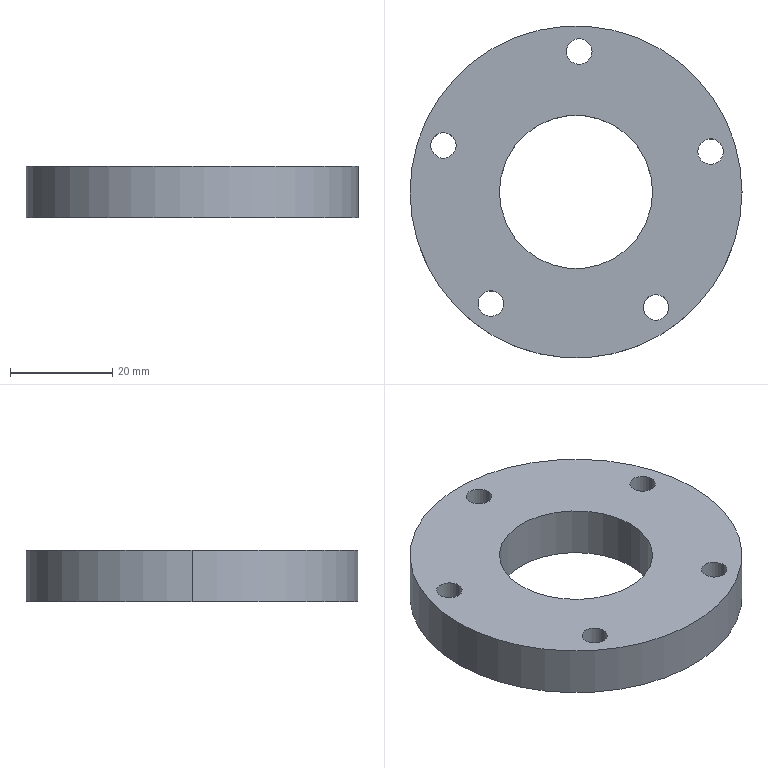Part | SolidWorks | features BaseBody 1 | 1 solid | 16 faces | box 65 x 65 x 10 mm | volume 25133 mm3 | cylinder 14 | plane 2 | commonest cylinder face diameters 5 x10 30 x2 65 x2
STEP:
#1=CARTESIAN_POINT('',(-23.45,9.102,10.));
#2=VERTEX_POINT('',#1);
#3=CARTESIAN_POINT('',(-28.45,9.102,10.));
#4=VERTEX_POINT('',#3);
#5=CARTESIAN_POINT('',(-25.95,9.102,10.));
#6=DIRECTION('',(0.,0.,-1.));
#7=DIRECTION('',(-1.,0.,0.));
#8=AXIS2_PLACEMENT_3D('',#5,#6,#7);
#9=CIRCLE('',#8,2.5);
#10=EDGE_CURVE('',#2,#4,#9,.T.);
#11=ORIENTED_EDGE('',*,*,#10,.F.);
#12=CARTESIAN_POINT('',(-23.45,9.102,0.));
#13=VERTEX_POINT('',#12);
#14=CARTESIAN_POINT('',(-23.45,9.102,10.));
#15=DIRECTION('',(0.,0.,-1.));
#16=VECTOR('',#15,1000.);
#17=LINE('',#14,#16);
#18=EDGE_CURVE('',#2,#13,#17,.T.);
#19=ORIENTED_EDGE('',*,*,#18,.T.);
#20=CARTESIAN_POINT('',(-28.45,9.102,0.));
#21=VERTEX_POINT('',#20);
#22=CARTESIAN_POINT('',(-25.95,9.102,0.));
#23=DIRECTION('',(0.,0.,1.));
#24=DIRECTION('',(-1.,0.,0.));
#25=AXIS2_PLACEMENT_3D('',#22,#23,#24);
#26=CIRCLE('',#25,2.5);
#27=EDGE_CURVE('',#21,#13,#26,.T.);
#28=ORIENTED_EDGE('',*,*,#27,.F.);
#29=CARTESIAN_POINT('',(-28.45,9.102,10.));
#30=DIRECTION('',(0.,0.,-1.));
#31=VECTOR('',#30,1000.);
#32=LINE('',#29,#31);
#33=EDGE_CURVE('',#4,#21,#32,.T.);
#34=ORIENTED_EDGE('',*,*,#33,.F.);
#35=EDGE_LOOP('',(#11,#19,#28,#34));
#36=FACE_OUTER_BOUND('',#35,.T.);
#37=CARTESIAN_POINT('',(-25.95,9.102,10.));
#38=DIRECTION('',(0.,0.,-1.));
#39=DIRECTION('',(-1.,0.,0.));
#40=AXIS2_PLACEMENT_3D('',#37,#38,#39);
#41=CYLINDRICAL_SURFACE('',#40,2.5);
#42=ADVANCED_FACE('',(#36),#41,.F.);
#43=CARTESIAN_POINT('',(18.144,-22.616,10.));
#44=VERTEX_POINT('',#43);
#45=CARTESIAN_POINT('',(13.144,-22.616,10.));
#46=VERTEX_POINT('',#45);
#47=CARTESIAN_POINT('',(15.644,-22.616,10.));
#48=DIRECTION('',(0.,0.,-1.));
#49=DIRECTION('',(-1.,0.,0.));
#50=AXIS2_PLACEMENT_3D('',#47,#48,#49);
#51=CIRCLE('',#50,2.5);
#52=EDGE_CURVE('',#44,#46,#51,.T.);
#53=ORIENTED_EDGE('',*,*,#52,.F.);
#54=CARTESIAN_POINT('',(18.144,-22.616,0.));
#55=VERTEX_POINT('',#54);
#56=CARTESIAN_POINT('',(18.144,-22.616,10.));
#57=DIRECTION('',(0.,0.,-1.));
#58=VECTOR('',#57,1000.);
#59=LINE('',#56,#58);
#60=EDGE_CURVE('',#44,#55,#59,.T.);
#61=ORIENTED_EDGE('',*,*,#60,.T.);
#62=CARTESIAN_POINT('',(13.144,-22.616,0.));
#63=VERTEX_POINT('',#62);
#64=CARTESIAN_POINT('',(15.644,-22.616,0.));
#65=DIRECTION('',(0.,0.,1.));
#66=DIRECTION('',(-1.,0.,0.));
#67=AXIS2_PLACEMENT_3D('',#64,#65,#66);
#68=CIRCLE('',#67,2.5);
#69=EDGE_CURVE('',#63,#55,#68,.T.);
#70=ORIENTED_EDGE('',*,*,#69,.F.);
#71=CARTESIAN_POINT('',(13.144,-22.616,10.));
#72=DIRECTION('',(0.,0.,-1.));
#73=VECTOR('',#72,1000.);
#74=LINE('',#71,#73);
#75=EDGE_CURVE('',#46,#63,#74,.T.);
#76=ORIENTED_EDGE('',*,*,#75,.F.);
#77=EDGE_LOOP('',(#53,#61,#70,#76));
#78=FACE_OUTER_BOUND('',#77,.T.);
#79=CARTESIAN_POINT('',(15.644,-22.616,10.));
#80=DIRECTION('',(0.,0.,-1.));
#81=DIRECTION('',(-1.,0.,0.));
#82=AXIS2_PLACEMENT_3D('',#79,#80,#81);
#83=CYLINDRICAL_SURFACE('',#82,2.5);
#84=ADVANCED_FACE('',(#78),#83,.F.);
#85=CARTESIAN_POINT('',(3.137,27.493,10.));
#86=VERTEX_POINT('',#85);
#87=CARTESIAN_POINT('',(-1.863,27.493,10.));
#88=VERTEX_POINT('',#87);
#89=CARTESIAN_POINT('',(0.637,27.493,10.));
#90=DIRECTION('',(0.,0.,-1.));
#91=DIRECTION('',(-1.,0.,0.));
#92=AXIS2_PLACEMENT_3D('',#89,#90,#91);
#93=CIRCLE('',#92,2.5);
#94=EDGE_CURVE('',#86,#88,#93,.T.);
#95=ORIENTED_EDGE('',*,*,#94,.F.);
#96=CARTESIAN_POINT('',(3.137,27.493,0.));
#97=VERTEX_POINT('',#96);
#98=CARTESIAN_POINT('',(3.137,27.493,10.));
#99=DIRECTION('',(0.,0.,-1.));
#100=VECTOR('',#99,1000.);
#101=LINE('',#98,#100);
#102=EDGE_CURVE('',#86,#97,#101,.T.);
#103=ORIENTED_EDGE('',*,*,#102,.T.);
#104=CARTESIAN_POINT('',(-1.863,27.493,0.));
#105=VERTEX_POINT('',#104);
#106=CARTESIAN_POINT('',(0.637,27.493,0.));
#107=DIRECTION('',(0.,0.,1.));
#108=DIRECTION('',(-1.,0.,0.));
#109=AXIS2_PLACEMENT_3D('',#106,#107,#108);
#110=CIRCLE('',#109,2.5);
#111=EDGE_CURVE('',#105,#97,#110,.T.);
#112=ORIENTED_EDGE('',*,*,#111,.F.);
#113=CARTESIAN_POINT('',(-1.863,27.493,10.));
#114=DIRECTION('',(0.,0.,-1.));
#115=VECTOR('',#114,1000.);
#116=LINE('',#113,#115);
#117=EDGE_CURVE('',#88,#105,#116,.T.);
#118=ORIENTED_EDGE('',*,*,#117,.F.);
#119=EDGE_LOOP('',(#95,#103,#112,#118));
#120=FACE_OUTER_BOUND('',#119,.T.);
#121=CARTESIAN_POINT('',(0.637,27.493,10.));
#122=DIRECTION('',(0.,0.,-1.));
#123=DIRECTION('',(-1.,0.,0.));
#124=AXIS2_PLACEMENT_3D('',#121,#122,#123);
#125=CYLINDRICAL_SURFACE('',#124,2.5);
#126=ADVANCED_FACE('',(#120),#125,.F.);
#127=CARTESIAN_POINT('',(32.5,0.,10.));
#128=VERTEX_POINT('',#127);
#129=CARTESIAN_POINT('',(-32.5,0.,10.));
#130=VERTEX_POINT('',#129);
#131=CARTESIAN_POINT('',(0.,0.,10.));
#132=DIRECTION('',(0.,0.,1.));
#133=DIRECTION('',(-1.,0.,0.));
#134=AXIS2_PLACEMENT_3D('',#131,#132,#133);
#135=CIRCLE('',#134,32.5);
#136=EDGE_CURVE('',#128,#130,#135,.T.);
#137=ORIENTED_EDGE('',*,*,#136,.F.);
#138=CARTESIAN_POINT('',(32.5,0.,0.));
#139=VERTEX_POINT('',#138);
#140=CARTESIAN_POINT('',(32.5,0.,10.));
#141=DIRECTION('',(0.,0.,-1.));
#142=VECTOR('',#141,1000.);
#143=LINE('',#140,#142);
#144=EDGE_CURVE('',#128,#139,#143,.T.);
#145=ORIENTED_EDGE('',*,*,#144,.T.);
#146=CARTESIAN_POINT('',(-32.5,0.,0.));
#147=VERTEX_POINT('',#146);
#148=CARTESIAN_POINT('',(0.,0.,0.));
#149=DIRECTION('',(0.,0.,1.));
#150=DIRECTION('',(-1.,0.,0.));
#151=AXIS2_PLACEMENT_3D('',#148,#149,#150);
#152=CIRCLE('',#151,32.5);
#153=EDGE_CURVE('',#139,#147,#152,.T.);
#154=ORIENTED_EDGE('',*,*,#153,.T.);
#155=CARTESIAN_POINT('',(-32.5,0.,10.));
#156=DIRECTION('',(0.,0.,-1.));
#157=VECTOR('',#156,1000.);
#158=LINE('',#155,#157);
#159=EDGE_CURVE('',#130,#147,#158,.T.);
#160=ORIENTED_EDGE('',*,*,#159,.F.);
#161=EDGE_LOOP('',(#137,#145,#154,#160));
#162=FACE_OUTER_BOUND('',#161,.T.);
#163=CARTESIAN_POINT('',(0.,0.,10.));
#164=DIRECTION('',(0.,0.,-1.));
#165=DIRECTION('',(-1.,0.,0.));
#166=AXIS2_PLACEMENT_3D('',#163,#164,#165);
#167=CYLINDRICAL_SURFACE('',#166,32.5);
#168=ADVANCED_FACE('',(#162),#167,.T.);
#169=CARTESIAN_POINT('',(15.,0.,10.));
#170=VERTEX_POINT('',#169);
#171=CARTESIAN_POINT('',(-15.,0.,10.));
#172=VERTEX_POINT('',#171);
#173=CARTESIAN_POINT('',(0.,0.,10.));
#174=DIRECTION('',(0.,0.,-1.));
#175=DIRECTION('',(-1.,0.,0.));
#176=AXIS2_PLACEMENT_3D('',#173,#174,#175);
#177=CIRCLE('',#176,15.);
#178=EDGE_CURVE('',#170,#172,#177,.T.);
#179=ORIENTED_EDGE('',*,*,#178,.F.);
#180=CARTESIAN_POINT('',(15.,0.,0.));
#181=VERTEX_POINT('',#180);
#182=CARTESIAN_POINT('',(15.,0.,10.));
#183=DIRECTION('',(0.,0.,-1.));
#184=VECTOR('',#183,1000.);
#185=LINE('',#182,#184);
#186=EDGE_CURVE('',#170,#181,#185,.T.);
#187=ORIENTED_EDGE('',*,*,#186,.T.);
#188=CARTESIAN_POINT('',(-15.,0.,0.));
#189=VERTEX_POINT('',#188);
#190=CARTESIAN_POINT('',(0.,0.,0.));
#191=DIRECTION('',(0.,0.,1.));
#192=DIRECTION('',(-1.,0.,0.));
#193=AXIS2_PLACEMENT_3D('',#190,#191,#192);
#194=CIRCLE('',#193,15.);
#195=EDGE_CURVE('',#189,#181,#194,.T.);
#196=ORIENTED_EDGE('',*,*,#195,.F.);
#197=CARTESIAN_POINT('',(-15.,0.,10.));
#198=DIRECTION('',(0.,0.,-1.));
#199=VECTOR('',#198,1000.);
#200=LINE('',#197,#199);
#201=EDGE_CURVE('',#172,#189,#200,.T.);
#202=ORIENTED_EDGE('',*,*,#201,.F.);
#203=EDGE_LOOP('',(#179,#187,#196,#202));
#204=FACE_OUTER_BOUND('',#203,.T.);
#205=CARTESIAN_POINT('',(0.,0.,10.));
#206=DIRECTION('',(0.,0.,-1.));
#207=DIRECTION('',(-1.,0.,0.));
#208=AXIS2_PLACEMENT_3D('',#205,#206,#207);
#209=CYLINDRICAL_SURFACE('',#208,15.);
#210=ADVANCED_FACE('',(#204),#209,.F.);
#211=CARTESIAN_POINT('',(28.844,7.89,10.));
#212=VERTEX_POINT('',#211);
#213=CARTESIAN_POINT('',(23.844,7.89,10.));
#214=VERTEX_POINT('',#213);
#215=CARTESIAN_POINT('',(26.344,7.89,10.));
#216=DIRECTION('',(0.,0.,-1.));
#217=DIRECTION('',(-1.,0.,0.));
#218=AXIS2_PLACEMENT_3D('',#215,#216,#217);
#219=CIRCLE('',#218,2.5);
#220=EDGE_CURVE('',#212,#214,#219,.T.);
#221=ORIENTED_EDGE('',*,*,#220,.F.);
#222=CARTESIAN_POINT('',(28.844,7.89,0.));
#223=VERTEX_POINT('',#222);
#224=CARTESIAN_POINT('',(28.844,7.89,10.));
#225=DIRECTION('',(0.,0.,-1.));
#226=VECTOR('',#225,1000.);
#227=LINE('',#224,#226);
#228=EDGE_CURVE('',#212,#223,#227,.T.);
#229=ORIENTED_EDGE('',*,*,#228,.T.);
#230=CARTESIAN_POINT('',(23.844,7.89,0.));
#231=VERTEX_POINT('',#230);
#232=CARTESIAN_POINT('',(26.344,7.89,0.));
#233=DIRECTION('',(0.,0.,1.));
#234=DIRECTION('',(-1.,0.,0.));
#235=AXIS2_PLACEMENT_3D('',#232,#233,#234);
#236=CIRCLE('',#235,2.5);
#237=EDGE_CURVE('',#231,#223,#236,.T.);
#238=ORIENTED_EDGE('',*,*,#237,.F.);
#239=CARTESIAN_POINT('',(23.844,7.89,10.));
#240=DIRECTION('',(0.,0.,-1.));
#241=VECTOR('',#240,1000.);
#242=LINE('',#239,#241);
#243=EDGE_CURVE('',#214,#231,#242,.T.);
#244=ORIENTED_EDGE('',*,*,#243,.F.);
#245=EDGE_LOOP('',(#221,#229,#238,#244));
#246=FACE_OUTER_BOUND('',#245,.T.);
#247=CARTESIAN_POINT('',(26.344,7.89,10.));
#248=DIRECTION('',(0.,0.,-1.));
#249=DIRECTION('',(-1.,0.,0.));
#250=AXIS2_PLACEMENT_3D('',#247,#248,#249);
#251=CYLINDRICAL_SURFACE('',#250,2.5);
#252=ADVANCED_FACE('',(#246),#251,.F.);
#253=CARTESIAN_POINT('',(-14.175,-21.868,10.));
#254=VERTEX_POINT('',#253);
#255=CARTESIAN_POINT('',(-19.175,-21.868,10.));
#256=VERTEX_POINT('',#255);
#257=CARTESIAN_POINT('',(-16.675,-21.868,10.));
#258=DIRECTION('',(0.,0.,-1.));
#259=DIRECTION('',(-1.,0.,0.));
#260=AXIS2_PLACEMENT_3D('',#257,#258,#259);
#261=CIRCLE('',#260,2.5);
#262=EDGE_CURVE('',#254,#256,#261,.T.);
#263=ORIENTED_EDGE('',*,*,#262,.F.);
#264=CARTESIAN_POINT('',(-14.175,-21.868,0.));
#265=VERTEX_POINT('',#264);
#266=CARTESIAN_POINT('',(-14.175,-21.868,10.));
#267=DIRECTION('',(0.,0.,-1.));
#268=VECTOR('',#267,1000.);
#269=LINE('',#266,#268);
#270=EDGE_CURVE('',#254,#265,#269,.T.);
#271=ORIENTED_EDGE('',*,*,#270,.T.);
#272=CARTESIAN_POINT('',(-19.175,-21.868,0.));
#273=VERTEX_POINT('',#272);
#274=CARTESIAN_POINT('',(-16.675,-21.868,0.));
#275=DIRECTION('',(0.,0.,1.));
#276=DIRECTION('',(-1.,0.,0.));
#277=AXIS2_PLACEMENT_3D('',#274,#275,#276);
#278=CIRCLE('',#277,2.5);
#279=EDGE_CURVE('',#273,#265,#278,.T.);
#280=ORIENTED_EDGE('',*,*,#279,.F.);
#281=CARTESIAN_POINT('',(-19.175,-21.868,10.));
#282=DIRECTION('',(0.,0.,-1.));
#283=VECTOR('',#282,1000.);
#284=LINE('',#281,#283);
#285=EDGE_CURVE('',#256,#273,#284,.T.);
#286=ORIENTED_EDGE('',*,*,#285,.F.);
#287=EDGE_LOOP('',(#263,#271,#280,#286));
#288=FACE_OUTER_BOUND('',#287,.T.);
#289=CARTESIAN_POINT('',(-16.675,-21.868,10.));
#290=DIRECTION('',(0.,0.,-1.));
#291=DIRECTION('',(-1.,0.,0.));
#292=AXIS2_PLACEMENT_3D('',#289,#290,#291);
#293=CYLINDRICAL_SURFACE('',#292,2.5);
#294=ADVANCED_FACE('',(#288),#293,.F.);
#295=CARTESIAN_POINT('',(-25.95,9.102,10.));
#296=DIRECTION('',(0.,0.,-1.));
#297=DIRECTION('',(-1.,0.,0.));
#298=AXIS2_PLACEMENT_3D('',#295,#296,#297);
#299=CIRCLE('',#298,2.5);
#300=EDGE_CURVE('',#4,#2,#299,.T.);
#301=ORIENTED_EDGE('',*,*,#300,.T.);
#302=ORIENTED_EDGE('',*,*,#10,.T.);
#303=EDGE_LOOP('',(#301,#302));
#304=FACE_BOUND('',#303,.T.);
#305=CARTESIAN_POINT('',(15.644,-22.616,10.));
#306=DIRECTION('',(0.,0.,-1.));
#307=DIRECTION('',(-1.,0.,0.));
#308=AXIS2_PLACEMENT_3D('',#305,#306,#307);
#309=CIRCLE('',#308,2.5);
#310=EDGE_CURVE('',#46,#44,#309,.T.);
#311=ORIENTED_EDGE('',*,*,#310,.T.);
#312=ORIENTED_EDGE('',*,*,#52,.T.);
#313=EDGE_LOOP('',(#311,#312));
#314=FACE_BOUND('',#313,.T.);
#315=CARTESIAN_POINT('',(0.637,27.493,10.));
#316=DIRECTION('',(0.,0.,-1.));
#317=DIRECTION('',(-1.,0.,0.));
#318=AXIS2_PLACEMENT_3D('',#315,#316,#317);
#319=CIRCLE('',#318,2.5);
#320=EDGE_CURVE('',#88,#86,#319,.T.);
#321=ORIENTED_EDGE('',*,*,#320,.T.);
#322=ORIENTED_EDGE('',*,*,#94,.T.);
#323=EDGE_LOOP('',(#321,#322));
#324=FACE_BOUND('',#323,.T.);
#325=CARTESIAN_POINT('',(0.,0.,10.));
#326=DIRECTION('',(0.,0.,1.));
#327=DIRECTION('',(-1.,0.,0.));
#328=AXIS2_PLACEMENT_3D('',#325,#326,#327);
#329=CIRCLE('',#328,32.5);
#330=EDGE_CURVE('',#130,#128,#329,.T.);
#331=ORIENTED_EDGE('',*,*,#330,.T.);
#332=ORIENTED_EDGE('',*,*,#136,.T.);
#333=EDGE_LOOP('',(#331,#332));
#334=FACE_OUTER_BOUND('',#333,.T.);
#335=CARTESIAN_POINT('',(0.,0.,10.));
#336=DIRECTION('',(0.,0.,-1.));
#337=DIRECTION('',(-1.,0.,0.));
#338=AXIS2_PLACEMENT_3D('',#335,#336,#337);
#339=CIRCLE('',#338,15.);
#340=EDGE_CURVE('',#172,#170,#339,.T.);
#341=ORIENTED_EDGE('',*,*,#340,.T.);
#342=ORIENTED_EDGE('',*,*,#178,.T.);
#343=EDGE_LOOP('',(#341,#342));
#344=FACE_BOUND('',#343,.T.);
#345=CARTESIAN_POINT('',(26.344,7.89,10.));
#346=DIRECTION('',(0.,0.,-1.));
#347=DIRECTION('',(-1.,0.,0.));
#348=AXIS2_PLACEMENT_3D('',#345,#346,#347);
#349=CIRCLE('',#348,2.5);
#350=EDGE_CURVE('',#214,#212,#349,.T.);
#351=ORIENTED_EDGE('',*,*,#350,.T.);
#352=ORIENTED_EDGE('',*,*,#220,.T.);
#353=EDGE_LOOP('',(#351,#352));
#354=FACE_BOUND('',#353,.T.);
#355=CARTESIAN_POINT('',(-16.675,-21.868,10.));
#356=DIRECTION('',(0.,0.,-1.));
#357=DIRECTION('',(-1.,0.,0.));
#358=AXIS2_PLACEMENT_3D('',#355,#356,#357);
#359=CIRCLE('',#358,2.5);
#360=EDGE_CURVE('',#256,#254,#359,.T.);
#361=ORIENTED_EDGE('',*,*,#360,.T.);
#362=ORIENTED_EDGE('',*,*,#262,.T.);
#363=EDGE_LOOP('',(#361,#362));
#364=FACE_BOUND('',#363,.T.);
#365=CARTESIAN_POINT('',(0.,0.,10.));
#366=DIRECTION('',(0.,0.,1.));
#367=DIRECTION('',(1.,0.,0.));
#368=AXIS2_PLACEMENT_3D('',#365,#366,#367);
#369=PLANE('',#368);
#370=ADVANCED_FACE('',(#304,#314,#324,#334,#344,#354,#364),#369,.T.);
#371=ORIENTED_EDGE('',*,*,#18,.F.);
#372=ORIENTED_EDGE('',*,*,#300,.F.);
#373=ORIENTED_EDGE('',*,*,#33,.T.);
#374=CARTESIAN_POINT('',(-25.95,9.102,0.));
#375=DIRECTION('',(0.,0.,1.));
#376=DIRECTION('',(-1.,0.,0.));
#377=AXIS2_PLACEMENT_3D('',#374,#375,#376);
#378=CIRCLE('',#377,2.5);
#379=EDGE_CURVE('',#13,#21,#378,.T.);
#380=ORIENTED_EDGE('',*,*,#379,.F.);
#381=EDGE_LOOP('',(#371,#372,#373,#380));
#382=FACE_OUTER_BOUND('',#381,.T.);
#383=CARTESIAN_POINT('',(-25.95,9.102,10.));
#384=DIRECTION('',(0.,0.,-1.));
#385=DIRECTION('',(-1.,0.,0.));
#386=AXIS2_PLACEMENT_3D('',#383,#384,#385);
#387=CYLINDRICAL_SURFACE('',#386,2.5);
#388=ADVANCED_FACE('',(#382),#387,.F.);
#389=ORIENTED_EDGE('',*,*,#60,.F.);
#390=ORIENTED_EDGE('',*,*,#310,.F.);
#391=ORIENTED_EDGE('',*,*,#75,.T.);
#392=CARTESIAN_POINT('',(15.644,-22.616,0.));
#393=DIRECTION('',(0.,0.,1.));
#394=DIRECTION('',(-1.,0.,0.));
#395=AXIS2_PLACEMENT_3D('',#392,#393,#394);
#396=CIRCLE('',#395,2.5);
#397=EDGE_CURVE('',#55,#63,#396,.T.);
#398=ORIENTED_EDGE('',*,*,#397,.F.);
#399=EDGE_LOOP('',(#389,#390,#391,#398));
#400=FACE_OUTER_BOUND('',#399,.T.);
#401=CARTESIAN_POINT('',(15.644,-22.616,10.));
#402=DIRECTION('',(0.,0.,-1.));
#403=DIRECTION('',(-1.,0.,0.));
#404=AXIS2_PLACEMENT_3D('',#401,#402,#403);
#405=CYLINDRICAL_SURFACE('',#404,2.5);
#406=ADVANCED_FACE('',(#400),#405,.F.);
#407=ORIENTED_EDGE('',*,*,#102,.F.);
#408=ORIENTED_EDGE('',*,*,#320,.F.);
#409=ORIENTED_EDGE('',*,*,#117,.T.);
#410=CARTESIAN_POINT('',(0.637,27.493,0.));
#411=DIRECTION('',(0.,0.,1.));
#412=DIRECTION('',(-1.,0.,0.));
#413=AXIS2_PLACEMENT_3D('',#410,#411,#412);
#414=CIRCLE('',#413,2.5);
#415=EDGE_CURVE('',#97,#105,#414,.T.);
#416=ORIENTED_EDGE('',*,*,#415,.F.);
#417=EDGE_LOOP('',(#407,#408,#409,#416));
#418=FACE_OUTER_BOUND('',#417,.T.);
#419=CARTESIAN_POINT('',(0.637,27.493,10.));
#420=DIRECTION('',(0.,0.,-1.));
#421=DIRECTION('',(-1.,0.,0.));
#422=AXIS2_PLACEMENT_3D('',#419,#420,#421);
#423=CYLINDRICAL_SURFACE('',#422,2.5);
#424=ADVANCED_FACE('',(#418),#423,.F.);
#425=ORIENTED_EDGE('',*,*,#144,.F.);
#426=ORIENTED_EDGE('',*,*,#330,.F.);
#427=ORIENTED_EDGE('',*,*,#159,.T.);
#428=CARTESIAN_POINT('',(0.,0.,0.));
#429=DIRECTION('',(0.,0.,1.));
#430=DIRECTION('',(-1.,0.,0.));
#431=AXIS2_PLACEMENT_3D('',#428,#429,#430);
#432=CIRCLE('',#431,32.5);
#433=EDGE_CURVE('',#147,#139,#432,.T.);
#434=ORIENTED_EDGE('',*,*,#433,.T.);
#435=EDGE_LOOP('',(#425,#426,#427,#434));
#436=FACE_OUTER_BOUND('',#435,.T.);
#437=CARTESIAN_POINT('',(0.,0.,10.));
#438=DIRECTION('',(0.,0.,-1.));
#439=DIRECTION('',(-1.,0.,0.));
#440=AXIS2_PLACEMENT_3D('',#437,#438,#439);
#441=CYLINDRICAL_SURFACE('',#440,32.5);
#442=ADVANCED_FACE('',(#436),#441,.T.);
#443=ORIENTED_EDGE('',*,*,#186,.F.);
#444=ORIENTED_EDGE('',*,*,#340,.F.);
#445=ORIENTED_EDGE('',*,*,#201,.T.);
#446=CARTESIAN_POINT('',(0.,0.,0.));
#447=DIRECTION('',(0.,0.,1.));
#448=DIRECTION('',(-1.,0.,0.));
#449=AXIS2_PLACEMENT_3D('',#446,#447,#448);
#450=CIRCLE('',#449,15.);
#451=EDGE_CURVE('',#181,#189,#450,.T.);
#452=ORIENTED_EDGE('',*,*,#451,.F.);
#453=EDGE_LOOP('',(#443,#444,#445,#452));
#454=FACE_OUTER_BOUND('',#453,.T.);
#455=CARTESIAN_POINT('',(0.,0.,10.));
#456=DIRECTION('',(0.,0.,-1.));
#457=DIRECTION('',(-1.,0.,0.));
#458=AXIS2_PLACEMENT_3D('',#455,#456,#457);
#459=CYLINDRICAL_SURFACE('',#458,15.);
#460=ADVANCED_FACE('',(#454),#459,.F.);
#461=ORIENTED_EDGE('',*,*,#228,.F.);
#462=ORIENTED_EDGE('',*,*,#350,.F.);
#463=ORIENTED_EDGE('',*,*,#243,.T.);
#464=CARTESIAN_POINT('',(26.344,7.89,0.));
#465=DIRECTION('',(0.,0.,1.));
#466=DIRECTION('',(-1.,0.,0.));
#467=AXIS2_PLACEMENT_3D('',#464,#465,#466);
#468=CIRCLE('',#467,2.5);
#469=EDGE_CURVE('',#223,#231,#468,.T.);
#470=ORIENTED_EDGE('',*,*,#469,.F.);
#471=EDGE_LOOP('',(#461,#462,#463,#470));
#472=FACE_OUTER_BOUND('',#471,.T.);
#473=CARTESIAN_POINT('',(26.344,7.89,10.));
#474=DIRECTION('',(0.,0.,-1.));
#475=DIRECTION('',(-1.,0.,0.));
#476=AXIS2_PLACEMENT_3D('',#473,#474,#475);
#477=CYLINDRICAL_SURFACE('',#476,2.5);
#478=ADVANCED_FACE('',(#472),#477,.F.);
#479=ORIENTED_EDGE('',*,*,#270,.F.);
#480=ORIENTED_EDGE('',*,*,#360,.F.);
#481=ORIENTED_EDGE('',*,*,#285,.T.);
#482=CARTESIAN_POINT('',(-16.675,-21.868,0.));
#483=DIRECTION('',(0.,0.,1.));
#484=DIRECTION('',(-1.,0.,0.));
#485=AXIS2_PLACEMENT_3D('',#482,#483,#484);
#486=CIRCLE('',#485,2.5);
#487=EDGE_CURVE('',#265,#273,#486,.T.);
#488=ORIENTED_EDGE('',*,*,#487,.F.);
#489=EDGE_LOOP('',(#479,#480,#481,#488));
#490=FACE_OUTER_BOUND('',#489,.T.);
#491=CARTESIAN_POINT('',(-16.675,-21.868,10.));
#492=DIRECTION('',(0.,0.,-1.));
#493=DIRECTION('',(-1.,0.,0.));
#494=AXIS2_PLACEMENT_3D('',#491,#492,#493);
#495=CYLINDRICAL_SURFACE('',#494,2.5);
#496=ADVANCED_FACE('',(#490),#495,.F.);
#497=ORIENTED_EDGE('',*,*,#27,.T.);
#498=ORIENTED_EDGE('',*,*,#379,.T.);
#499=EDGE_LOOP('',(#497,#498));
#500=FACE_BOUND('',#499,.T.);
#501=ORIENTED_EDGE('',*,*,#279,.T.);
#502=ORIENTED_EDGE('',*,*,#487,.T.);
#503=EDGE_LOOP('',(#501,#502));
#504=FACE_BOUND('',#503,.T.);
#505=ORIENTED_EDGE('',*,*,#69,.T.);
#506=ORIENTED_EDGE('',*,*,#397,.T.);
#507=EDGE_LOOP('',(#505,#506));
#508=FACE_BOUND('',#507,.T.);
#509=ORIENTED_EDGE('',*,*,#237,.T.);
#510=ORIENTED_EDGE('',*,*,#469,.T.);
#511=EDGE_LOOP('',(#509,#510));
#512=FACE_BOUND('',#511,.T.);
#513=ORIENTED_EDGE('',*,*,#111,.T.);
#514=ORIENTED_EDGE('',*,*,#415,.T.);
#515=EDGE_LOOP('',(#513,#514));
#516=FACE_BOUND('',#515,.T.);
#517=ORIENTED_EDGE('',*,*,#195,.T.);
#518=ORIENTED_EDGE('',*,*,#451,.T.);
#519=EDGE_LOOP('',(#517,#518));
#520=FACE_BOUND('',#519,.T.);
#521=ORIENTED_EDGE('',*,*,#433,.F.);
#522=ORIENTED_EDGE('',*,*,#153,.F.);
#523=EDGE_LOOP('',(#521,#522));
#524=FACE_OUTER_BOUND('',#523,.T.);
#525=CARTESIAN_POINT('',(0.,0.,0.));
#526=DIRECTION('',(0.,0.,1.));
#527=DIRECTION('',(1.,0.,0.));
#528=AXIS2_PLACEMENT_3D('',#525,#526,#527);
#529=PLANE('',#528);
#530=ADVANCED_FACE('',(#500,#504,#508,#512,#516,#520,#524),#529,.F.);
#531=CLOSED_SHELL('',(#42,#84,#126,#168,#210,#252,#294,#370,#388,#406,#424,#442,#460,#478,#496,#530));
#532=MANIFOLD_SOLID_BREP('',#531);
#533=CARTESIAN_POINT('',(0.,0.,0.));
#534=DIRECTION('',(0.,0.,1.));
#535=DIRECTION('',(1.,0.,0.));
#536=AXIS2_PLACEMENT_3D('',#533,#534,#535);
#537=(LENGTH_UNIT()NAMED_UNIT(*)SI_UNIT(.MILLI.,.METRE.));
#538=UNCERTAINTY_MEASURE_WITH_UNIT(LENGTH_MEASURE(0.00001),#537,'','');
#539=(NAMED_UNIT(*)PLANE_ANGLE_UNIT()SI_UNIT($,.RADIAN.));
#540=(NAMED_UNIT(*)SI_UNIT($,.STERADIAN.)SOLID_ANGLE_UNIT());
#541=(GEOMETRIC_REPRESENTATION_CONTEXT(3)GLOBAL_UNCERTAINTY_ASSIGNED_CONTEXT((#538))GLOBAL_UNIT_ASSIGNED_CONTEXT((#537,#539,#540))REPRESENTATION_CONTEXT('',''));
#542=ADVANCED_BREP_SHAPE_REPRESENTATION('',(#532,#536),#541);